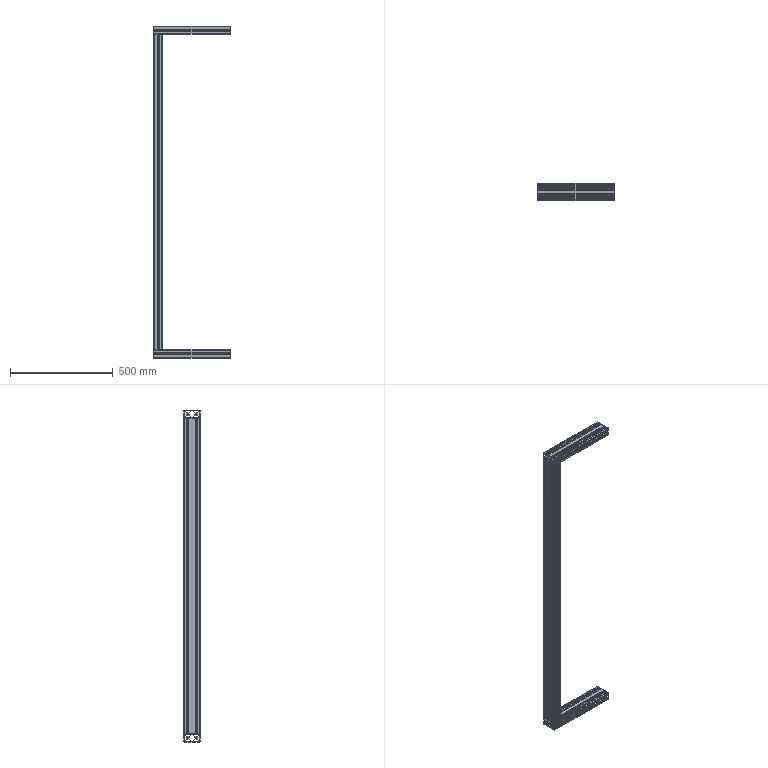Part | SolidWorks | features WeldCornerFeat 2, WeldMemberFeat 2, WeldmentFeature 1 | 3 solids | 465 faces | box 370 x 80 x 1615 mm | volume 2239494 mm3 | plane 426 | cylinder 39 | commonest cylinder face diameters 9 x15 5 x12 6.8 x12